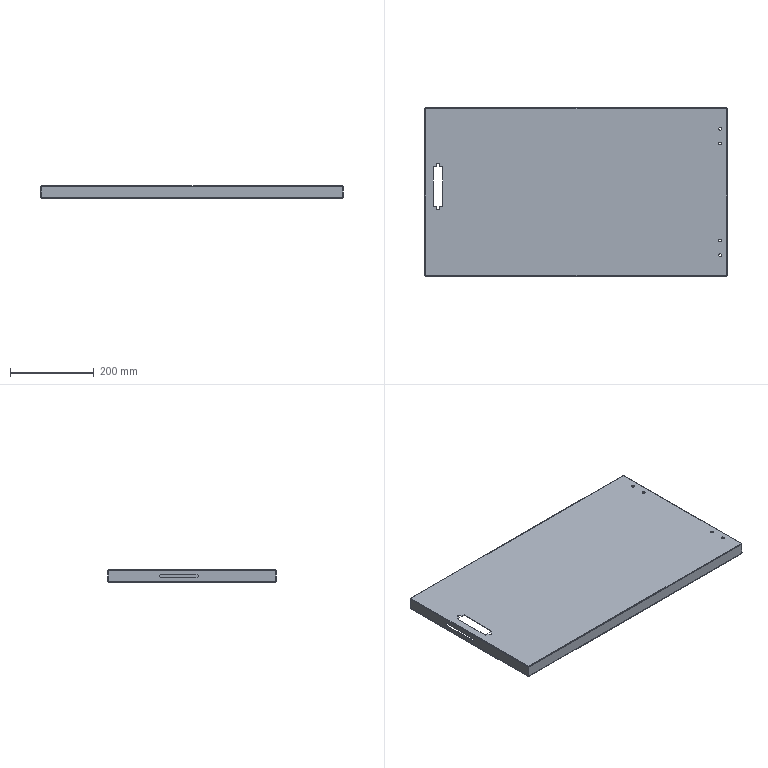Part | 1 solid | 95 faces | box 723 x 402 x 30 mm | volume 447828 mm3 | plane 50 | cylinder 29 | spline 16 | commonest cylinder face diameters 7 x13 1.473 x8 3.873 x8